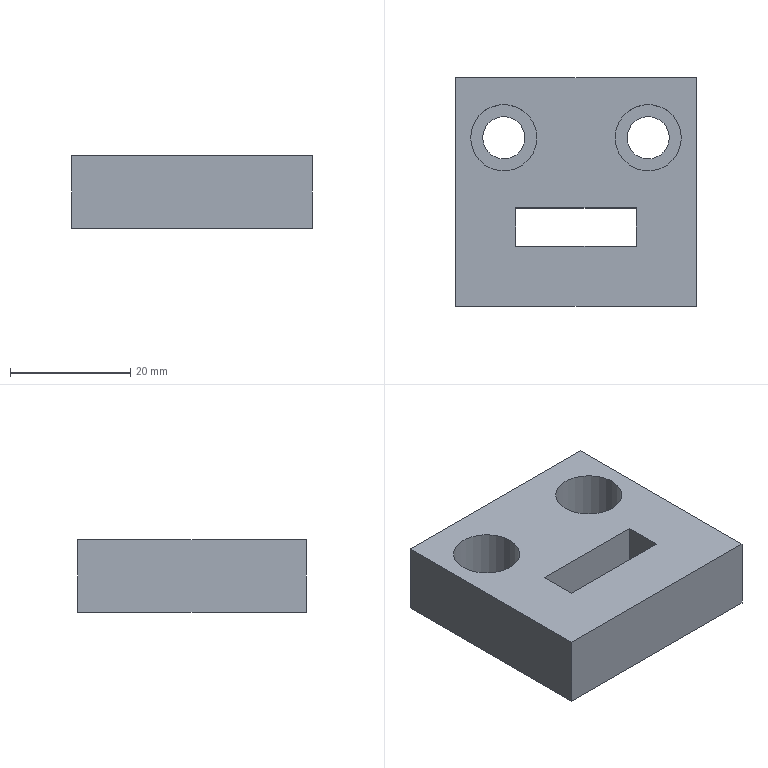Part | STEP file | lll_id714_x_t | 1 solid | 16 faces | box 40 x 38 x 12 mm | volume 14885 mm3 | plane 12 | cylinder 4 | commonest cylinder face diameters 7.009 x2 11.008 x2
STEP:
#1=CARTESIAN_POINT('',(295.5,-162.325,-12.));
#2=VERTEX_POINT('',#1);
#3=CARTESIAN_POINT('',(295.5,-168.675,-12.));
#4=VERTEX_POINT('',#3);
#5=CARTESIAN_POINT('',(295.5,-162.325,-12.));
#6=DIRECTION('',(0.,-1.,0.));
#7=VECTOR('',#6,1.);
#8=LINE('',#5,#7);
#9=EDGE_CURVE('',#2,#4,#8,.T.);
#10=ORIENTED_EDGE('',*,*,#9,.F.);
#11=CARTESIAN_POINT('',(275.5,-162.325,-12.));
#12=VERTEX_POINT('',#11);
#13=CARTESIAN_POINT('',(295.5,-162.325,-12.));
#14=DIRECTION('',(-1.,0.,0.));
#15=VECTOR('',#14,1.);
#16=LINE('',#13,#15);
#17=EDGE_CURVE('',#2,#12,#16,.T.);
#18=ORIENTED_EDGE('',*,*,#17,.T.);
#19=CARTESIAN_POINT('',(275.5,-168.675,-12.));
#20=VERTEX_POINT('',#19);
#21=CARTESIAN_POINT('',(275.5,-162.325,-12.));
#22=DIRECTION('',(0.,-1.,0.));
#23=VECTOR('',#22,1.);
#24=LINE('',#21,#23);
#25=EDGE_CURVE('',#12,#20,#24,.T.);
#26=ORIENTED_EDGE('',*,*,#25,.T.);
#27=CARTESIAN_POINT('',(295.5,-168.675,-12.));
#28=DIRECTION('',(-1.,0.,0.));
#29=VECTOR('',#28,1.);
#30=LINE('',#27,#29);
#31=EDGE_CURVE('',#4,#20,#30,.T.);
#32=ORIENTED_EDGE('',*,*,#31,.F.);
#33=EDGE_LOOP('',(#10,#18,#26,#32));
#34=FACE_BOUND('',#33,.T.);
#35=CARTESIAN_POINT('',(305.505,-140.675,-12.));
#36=VERTEX_POINT('',#35);
#37=CARTESIAN_POINT('',(305.505,-178.675,-12.));
#38=VERTEX_POINT('',#37);
#39=CARTESIAN_POINT('',(305.505,-165.5,-12.));
#40=DIRECTION('',(0.,-1.,0.));
#41=VECTOR('',#40,1.);
#42=LINE('',#39,#41);
#43=EDGE_CURVE('',#36,#38,#42,.T.);
#44=ORIENTED_EDGE('',*,*,#43,.T.);
#45=CARTESIAN_POINT('',(265.505,-178.675,-12.));
#46=VERTEX_POINT('',#45);
#47=CARTESIAN_POINT('',(0.,-178.675,-12.));
#48=DIRECTION('',(-1.,0.,0.));
#49=VECTOR('',#48,1.);
#50=LINE('',#47,#49);
#51=EDGE_CURVE('',#38,#46,#50,.T.);
#52=ORIENTED_EDGE('',*,*,#51,.T.);
#53=CARTESIAN_POINT('',(265.505,-140.675,-12.));
#54=VERTEX_POINT('',#53);
#55=CARTESIAN_POINT('',(265.505,-165.5,-12.));
#56=DIRECTION('',(0.,1.,0.));
#57=VECTOR('',#56,1.);
#58=LINE('',#55,#57);
#59=EDGE_CURVE('',#46,#54,#58,.T.);
#60=ORIENTED_EDGE('',*,*,#59,.T.);
#61=CARTESIAN_POINT('',(0.,-140.675,-12.));
#62=DIRECTION('',(1.,0.,0.));
#63=VECTOR('',#62,1.);
#64=LINE('',#61,#63);
#65=EDGE_CURVE('',#54,#36,#64,.T.);
#66=ORIENTED_EDGE('',*,*,#65,.T.);
#67=EDGE_LOOP('',(#44,#52,#60,#66));
#68=FACE_BOUND('',#67,.T.);
#69=CARTESIAN_POINT('',(277.009,-150.675,-12.));
#70=VERTEX_POINT('',#69);
#71=CARTESIAN_POINT('',(273.505,-150.675,-12.));
#72=DIRECTION('',(0.,0.,1.));
#73=DIRECTION('',(1.,0.,0.));
#74=AXIS2_PLACEMENT_3D('',#71,#72,#73);
#75=CIRCLE('',#74,3.505);
#76=EDGE_CURVE('',#70,#70,#75,.T.);
#77=ORIENTED_EDGE('',*,*,#76,.T.);
#78=EDGE_LOOP('',(#77));
#79=FACE_BOUND('',#78,.T.);
#80=CARTESIAN_POINT('',(294.,-150.675,-12.));
#81=VERTEX_POINT('',#80);
#82=CARTESIAN_POINT('',(297.505,-150.675,-12.));
#83=DIRECTION('',(0.,0.,-1.));
#84=DIRECTION('',(-1.,0.,0.));
#85=AXIS2_PLACEMENT_3D('',#82,#83,#84);
#86=CIRCLE('',#85,3.505);
#87=EDGE_CURVE('',#81,#81,#86,.T.);
#88=ORIENTED_EDGE('',*,*,#87,.F.);
#89=EDGE_LOOP('',(#88));
#90=FACE_BOUND('',#89,.T.);
#91=CARTESIAN_POINT('',(285.505,-165.5,-12.));
#92=DIRECTION('',(0.,0.,-1.));
#93=DIRECTION('',(1.,0.,0.));
#94=AXIS2_PLACEMENT_3D('',#91,#92,#93);
#95=PLANE('',#94);
#96=ADVANCED_FACE('',(#34,#68,#79,#90),#95,.T.);
#97=CARTESIAN_POINT('',(305.505,-140.675,0.));
#98=VERTEX_POINT('',#97);
#99=CARTESIAN_POINT('',(265.505,-140.675,0.));
#100=VERTEX_POINT('',#99);
#101=CARTESIAN_POINT('',(0.,-140.675,0.));
#102=DIRECTION('',(-1.,0.,0.));
#103=VECTOR('',#102,1.);
#104=LINE('',#101,#103);
#105=EDGE_CURVE('',#98,#100,#104,.T.);
#106=ORIENTED_EDGE('',*,*,#105,.T.);
#107=CARTESIAN_POINT('',(265.505,-178.675,0.));
#108=VERTEX_POINT('',#107);
#109=CARTESIAN_POINT('',(265.505,-165.5,0.));
#110=DIRECTION('',(0.,-1.,0.));
#111=VECTOR('',#110,1.);
#112=LINE('',#109,#111);
#113=EDGE_CURVE('',#100,#108,#112,.T.);
#114=ORIENTED_EDGE('',*,*,#113,.T.);
#115=CARTESIAN_POINT('',(305.505,-178.675,0.));
#116=VERTEX_POINT('',#115);
#117=CARTESIAN_POINT('',(0.,-178.675,0.));
#118=DIRECTION('',(1.,0.,0.));
#119=VECTOR('',#118,1.);
#120=LINE('',#117,#119);
#121=EDGE_CURVE('',#108,#116,#120,.T.);
#122=ORIENTED_EDGE('',*,*,#121,.T.);
#123=CARTESIAN_POINT('',(305.505,-165.5,0.));
#124=DIRECTION('',(0.,1.,0.));
#125=VECTOR('',#124,1.);
#126=LINE('',#123,#125);
#127=EDGE_CURVE('',#116,#98,#126,.T.);
#128=ORIENTED_EDGE('',*,*,#127,.T.);
#129=EDGE_LOOP('',(#106,#114,#122,#128));
#130=FACE_BOUND('',#129,.T.);
#131=CARTESIAN_POINT('',(295.5,-168.675,0.));
#132=VERTEX_POINT('',#131);
#133=CARTESIAN_POINT('',(275.5,-168.675,0.));
#134=VERTEX_POINT('',#133);
#135=CARTESIAN_POINT('',(295.5,-168.675,0.));
#136=DIRECTION('',(-1.,0.,0.));
#137=VECTOR('',#136,1.);
#138=LINE('',#135,#137);
#139=EDGE_CURVE('',#132,#134,#138,.T.);
#140=ORIENTED_EDGE('',*,*,#139,.T.);
#141=CARTESIAN_POINT('',(275.5,-162.325,0.));
#142=VERTEX_POINT('',#141);
#143=CARTESIAN_POINT('',(275.5,-162.325,0.));
#144=DIRECTION('',(0.,-1.,0.));
#145=VECTOR('',#144,1.);
#146=LINE('',#143,#145);
#147=EDGE_CURVE('',#142,#134,#146,.T.);
#148=ORIENTED_EDGE('',*,*,#147,.F.);
#149=CARTESIAN_POINT('',(295.5,-162.325,0.));
#150=VERTEX_POINT('',#149);
#151=CARTESIAN_POINT('',(295.5,-162.325,0.));
#152=DIRECTION('',(-1.,0.,0.));
#153=VECTOR('',#152,1.);
#154=LINE('',#151,#153);
#155=EDGE_CURVE('',#150,#142,#154,.T.);
#156=ORIENTED_EDGE('',*,*,#155,.F.);
#157=CARTESIAN_POINT('',(295.5,-162.325,0.));
#158=DIRECTION('',(0.,-1.,0.));
#159=VECTOR('',#158,1.);
#160=LINE('',#157,#159);
#161=EDGE_CURVE('',#150,#132,#160,.T.);
#162=ORIENTED_EDGE('',*,*,#161,.T.);
#163=EDGE_LOOP('',(#140,#148,#156,#162));
#164=FACE_BOUND('',#163,.T.);
#165=CARTESIAN_POINT('',(279.009,-150.675,0.));
#166=VERTEX_POINT('',#165);
#167=CARTESIAN_POINT('',(273.505,-150.675,0.));
#168=DIRECTION('',(0.,0.,-1.));
#169=DIRECTION('',(1.,0.,0.));
#170=AXIS2_PLACEMENT_3D('',#167,#168,#169);
#171=CIRCLE('',#170,5.504);
#172=EDGE_CURVE('',#166,#166,#171,.T.);
#173=ORIENTED_EDGE('',*,*,#172,.T.);
#174=EDGE_LOOP('',(#173));
#175=FACE_BOUND('',#174,.T.);
#176=CARTESIAN_POINT('',(292.001,-150.675,0.));
#177=VERTEX_POINT('',#176);
#178=CARTESIAN_POINT('',(297.505,-150.675,0.));
#179=DIRECTION('',(0.,0.,1.));
#180=DIRECTION('',(-1.,0.,0.));
#181=AXIS2_PLACEMENT_3D('',#178,#179,#180);
#182=CIRCLE('',#181,5.504);
#183=EDGE_CURVE('',#177,#177,#182,.T.);
#184=ORIENTED_EDGE('',*,*,#183,.F.);
#185=EDGE_LOOP('',(#184));
#186=FACE_BOUND('',#185,.T.);
#187=CARTESIAN_POINT('',(285.505,-165.5,0.));
#188=DIRECTION('',(0.,0.,1.));
#189=DIRECTION('',(-1.,0.,0.));
#190=AXIS2_PLACEMENT_3D('',#187,#188,#189);
#191=PLANE('',#190);
#192=ADVANCED_FACE('',(#130,#164,#175,#186),#191,.T.);
#193=CARTESIAN_POINT('',(305.505,-140.675,0.));
#194=DIRECTION('',(0.,0.,1.));
#195=VECTOR('',#194,1.);
#196=LINE('',#193,#195);
#197=EDGE_CURVE('',#36,#98,#196,.T.);
#198=ORIENTED_EDGE('',*,*,#197,.F.);
#199=ORIENTED_EDGE('',*,*,#65,.F.);
#200=CARTESIAN_POINT('',(265.505,-140.675,-12.));
#201=DIRECTION('',(0.,0.,1.));
#202=VECTOR('',#201,1.);
#203=LINE('',#200,#202);
#204=EDGE_CURVE('',#54,#100,#203,.T.);
#205=ORIENTED_EDGE('',*,*,#204,.T.);
#206=ORIENTED_EDGE('',*,*,#105,.F.);
#207=EDGE_LOOP('',(#198,#199,#205,#206));
#208=FACE_OUTER_BOUND('',#207,.T.);
#209=CARTESIAN_POINT('',(0.,-140.675,0.));
#210=DIRECTION('',(0.,1.,0.));
#211=DIRECTION('',(0.,0.,1.));
#212=AXIS2_PLACEMENT_3D('',#209,#210,#211);
#213=PLANE('',#212);
#214=ADVANCED_FACE('',(#208),#213,.T.);
#215=ORIENTED_EDGE('',*,*,#204,.F.);
#216=ORIENTED_EDGE('',*,*,#59,.F.);
#217=CARTESIAN_POINT('',(265.505,-178.675,0.));
#218=DIRECTION('',(0.,0.,1.));
#219=VECTOR('',#218,1.);
#220=LINE('',#217,#219);
#221=EDGE_CURVE('',#46,#108,#220,.T.);
#222=ORIENTED_EDGE('',*,*,#221,.T.);
#223=ORIENTED_EDGE('',*,*,#113,.F.);
#224=EDGE_LOOP('',(#215,#216,#222,#223));
#225=FACE_OUTER_BOUND('',#224,.T.);
#226=CARTESIAN_POINT('',(265.505,-165.5,-12.));
#227=DIRECTION('',(-1.,0.,0.));
#228=DIRECTION('',(0.,0.,-1.));
#229=AXIS2_PLACEMENT_3D('',#226,#227,#228);
#230=PLANE('',#229);
#231=ADVANCED_FACE('',(#225),#230,.T.);
#232=ORIENTED_EDGE('',*,*,#221,.F.);
#233=ORIENTED_EDGE('',*,*,#51,.F.);
#234=CARTESIAN_POINT('',(305.505,-178.675,-12.));
#235=DIRECTION('',(0.,0.,1.));
#236=VECTOR('',#235,1.);
#237=LINE('',#234,#236);
#238=EDGE_CURVE('',#38,#116,#237,.T.);
#239=ORIENTED_EDGE('',*,*,#238,.T.);
#240=ORIENTED_EDGE('',*,*,#121,.F.);
#241=EDGE_LOOP('',(#232,#233,#239,#240));
#242=FACE_OUTER_BOUND('',#241,.T.);
#243=CARTESIAN_POINT('',(0.,-178.675,0.));
#244=DIRECTION('',(0.,1.,0.));
#245=DIRECTION('',(0.,0.,1.));
#246=AXIS2_PLACEMENT_3D('',#243,#244,#245);
#247=PLANE('',#246);
#248=ADVANCED_FACE('',(#242),#247,.F.);
#249=ORIENTED_EDGE('',*,*,#43,.F.);
#250=ORIENTED_EDGE('',*,*,#197,.T.);
#251=ORIENTED_EDGE('',*,*,#127,.F.);
#252=ORIENTED_EDGE('',*,*,#238,.F.);
#253=EDGE_LOOP('',(#249,#250,#251,#252));
#254=FACE_OUTER_BOUND('',#253,.T.);
#255=CARTESIAN_POINT('',(305.505,-165.5,-12.));
#256=DIRECTION('',(1.,0.,0.));
#257=DIRECTION('',(0.,0.,1.));
#258=AXIS2_PLACEMENT_3D('',#255,#256,#257);
#259=PLANE('',#258);
#260=ADVANCED_FACE('',(#254),#259,.T.);
#261=CARTESIAN_POINT('',(275.5,-168.675,-12.));
#262=DIRECTION('',(0.,0.,-1.));
#263=VECTOR('',#262,1.);
#264=LINE('',#261,#263);
#265=EDGE_CURVE('',#134,#20,#264,.T.);
#266=ORIENTED_EDGE('',*,*,#265,.T.);
#267=ORIENTED_EDGE('',*,*,#25,.F.);
#268=CARTESIAN_POINT('',(275.5,-162.325,-12.));
#269=DIRECTION('',(0.,0.,-1.));
#270=VECTOR('',#269,1.);
#271=LINE('',#268,#270);
#272=EDGE_CURVE('',#142,#12,#271,.T.);
#273=ORIENTED_EDGE('',*,*,#272,.F.);
#274=ORIENTED_EDGE('',*,*,#147,.T.);
#275=EDGE_LOOP('',(#266,#267,#273,#274));
#276=FACE_OUTER_BOUND('',#275,.T.);
#277=CARTESIAN_POINT('',(275.5,-162.325,-12.));
#278=DIRECTION('',(-1.,0.,0.));
#279=DIRECTION('',(0.,0.,-1.));
#280=AXIS2_PLACEMENT_3D('',#277,#278,#279);
#281=PLANE('',#280);
#282=ADVANCED_FACE('',(#276),#281,.F.);
#283=CARTESIAN_POINT('',(295.5,-168.675,-12.));
#284=DIRECTION('',(0.,0.,-1.));
#285=VECTOR('',#284,1.);
#286=LINE('',#283,#285);
#287=EDGE_CURVE('',#132,#4,#286,.T.);
#288=ORIENTED_EDGE('',*,*,#287,.F.);
#289=ORIENTED_EDGE('',*,*,#161,.F.);
#290=CARTESIAN_POINT('',(295.5,-162.325,-12.));
#291=DIRECTION('',(0.,0.,-1.));
#292=VECTOR('',#291,1.);
#293=LINE('',#290,#292);
#294=EDGE_CURVE('',#150,#2,#293,.T.);
#295=ORIENTED_EDGE('',*,*,#294,.T.);
#296=ORIENTED_EDGE('',*,*,#9,.T.);
#297=EDGE_LOOP('',(#288,#289,#295,#296));
#298=FACE_OUTER_BOUND('',#297,.T.);
#299=CARTESIAN_POINT('',(295.5,-162.325,-12.));
#300=DIRECTION('',(-1.,0.,0.));
#301=DIRECTION('',(0.,0.,-1.));
#302=AXIS2_PLACEMENT_3D('',#299,#300,#301);
#303=PLANE('',#302);
#304=ADVANCED_FACE('',(#298),#303,.T.);
#305=ORIENTED_EDGE('',*,*,#272,.T.);
#306=ORIENTED_EDGE('',*,*,#17,.F.);
#307=ORIENTED_EDGE('',*,*,#294,.F.);
#308=ORIENTED_EDGE('',*,*,#155,.T.);
#309=EDGE_LOOP('',(#305,#306,#307,#308));
#310=FACE_OUTER_BOUND('',#309,.T.);
#311=CARTESIAN_POINT('',(0.,-162.325,0.));
#312=DIRECTION('',(0.,1.,0.));
#313=DIRECTION('',(0.,0.,1.));
#314=AXIS2_PLACEMENT_3D('',#311,#312,#313);
#315=PLANE('',#314);
#316=ADVANCED_FACE('',(#310),#315,.F.);
#317=ORIENTED_EDGE('',*,*,#265,.F.);
#318=ORIENTED_EDGE('',*,*,#139,.F.);
#319=ORIENTED_EDGE('',*,*,#287,.T.);
#320=ORIENTED_EDGE('',*,*,#31,.T.);
#321=EDGE_LOOP('',(#317,#318,#319,#320));
#322=FACE_OUTER_BOUND('',#321,.T.);
#323=CARTESIAN_POINT('',(0.,-168.675,0.));
#324=DIRECTION('',(0.,1.,0.));
#325=DIRECTION('',(0.,0.,1.));
#326=AXIS2_PLACEMENT_3D('',#323,#324,#325);
#327=PLANE('',#326);
#328=ADVANCED_FACE('',(#322),#327,.T.);
#329=CARTESIAN_POINT('',(270.,-150.675,-8.));
#330=VERTEX_POINT('',#329);
#331=CARTESIAN_POINT('',(273.505,-150.675,-8.));
#332=DIRECTION('',(0.,0.,-1.));
#333=DIRECTION('',(-1.,0.,0.));
#334=AXIS2_PLACEMENT_3D('',#331,#332,#333);
#335=CIRCLE('',#334,3.505);
#336=EDGE_CURVE('',#330,#330,#335,.T.);
#337=ORIENTED_EDGE('',*,*,#336,.F.);
#338=EDGE_LOOP('',(#337));
#339=FACE_BOUND('',#338,.T.);
#340=ORIENTED_EDGE('',*,*,#76,.F.);
#341=EDGE_LOOP('',(#340));
#342=FACE_BOUND('',#341,.T.);
#343=CARTESIAN_POINT('',(273.505,-150.675,0.));
#344=DIRECTION('',(0.,0.,-1.));
#345=DIRECTION('',(-1.,0.,0.));
#346=AXIS2_PLACEMENT_3D('',#343,#344,#345);
#347=CYLINDRICAL_SURFACE('',#346,3.505);
#348=ADVANCED_FACE('',(#339,#342),#347,.F.);
#349=ORIENTED_EDGE('',*,*,#336,.T.);
#350=EDGE_LOOP('',(#349));
#351=FACE_BOUND('',#350,.T.);
#352=CARTESIAN_POINT('',(268.001,-150.675,-8.));
#353=VERTEX_POINT('',#352);
#354=CARTESIAN_POINT('',(273.505,-150.675,-8.));
#355=DIRECTION('',(0.,0.,-1.));
#356=DIRECTION('',(-1.,0.,0.));
#357=AXIS2_PLACEMENT_3D('',#354,#355,#356);
#358=CIRCLE('',#357,5.504);
#359=EDGE_CURVE('',#353,#353,#358,.T.);
#360=ORIENTED_EDGE('',*,*,#359,.F.);
#361=EDGE_LOOP('',(#360));
#362=FACE_BOUND('',#361,.T.);
#363=CARTESIAN_POINT('',(273.505,-150.675,-8.));
#364=DIRECTION('',(0.,0.,-1.));
#365=DIRECTION('',(-1.,0.,0.));
#366=AXIS2_PLACEMENT_3D('',#363,#364,#365);
#367=PLANE('',#366);
#368=ADVANCED_FACE('',(#351,#362),#367,.F.);
#369=ORIENTED_EDGE('',*,*,#359,.T.);
#370=EDGE_LOOP('',(#369));
#371=FACE_BOUND('',#370,.T.);
#372=ORIENTED_EDGE('',*,*,#172,.F.);
#373=EDGE_LOOP('',(#372));
#374=FACE_BOUND('',#373,.T.);
#375=CARTESIAN_POINT('',(273.505,-150.675,0.));
#376=DIRECTION('',(0.,0.,-1.));
#377=DIRECTION('',(-1.,0.,0.));
#378=AXIS2_PLACEMENT_3D('',#375,#376,#377);
#379=CYLINDRICAL_SURFACE('',#378,5.504);
#380=ADVANCED_FACE('',(#371,#374),#379,.F.);
#381=CARTESIAN_POINT('',(294.,-150.675,-8.));
#382=VERTEX_POINT('',#381);
#383=CARTESIAN_POINT('',(297.505,-150.675,-8.));
#384=DIRECTION('',(0.,0.,1.));
#385=DIRECTION('',(-1.,0.,0.));
#386=AXIS2_PLACEMENT_3D('',#383,#384,#385);
#387=CIRCLE('',#386,3.505);
#388=EDGE_CURVE('',#382,#382,#387,.T.);
#389=ORIENTED_EDGE('',*,*,#388,.T.);
#390=EDGE_LOOP('',(#389));
#391=FACE_BOUND('',#390,.T.);
#392=ORIENTED_EDGE('',*,*,#87,.T.);
#393=EDGE_LOOP('',(#392));
#394=FACE_BOUND('',#393,.T.);
#395=CARTESIAN_POINT('',(297.505,-150.675,0.));
#396=DIRECTION('',(0.,0.,-1.));
#397=DIRECTION('',(1.,0.,0.));
#398=AXIS2_PLACEMENT_3D('',#395,#396,#397);
#399=CYLINDRICAL_SURFACE('',#398,3.505);
#400=ADVANCED_FACE('',(#391,#394),#399,.F.);
#401=ORIENTED_EDGE('',*,*,#388,.F.);
#402=EDGE_LOOP('',(#401));
#403=FACE_BOUND('',#402,.T.);
#404=CARTESIAN_POINT('',(292.001,-150.675,-8.));
#405=VERTEX_POINT('',#404);
#406=CARTESIAN_POINT('',(297.505,-150.675,-8.));
#407=DIRECTION('',(0.,0.,1.));
#408=DIRECTION('',(-1.,0.,0.));
#409=AXIS2_PLACEMENT_3D('',#406,#407,#408);
#410=CIRCLE('',#409,5.504);
#411=EDGE_CURVE('',#405,#405,#410,.T.);
#412=ORIENTED_EDGE('',*,*,#411,.T.);
#413=EDGE_LOOP('',(#412));
#414=FACE_BOUND('',#413,.T.);
#415=CARTESIAN_POINT('',(297.505,-150.675,-8.));
#416=DIRECTION('',(0.,0.,-1.));
#417=DIRECTION('',(1.,0.,0.));
#418=AXIS2_PLACEMENT_3D('',#415,#416,#417);
#419=PLANE('',#418);
#420=ADVANCED_FACE('',(#403,#414),#419,.F.);
#421=ORIENTED_EDGE('',*,*,#411,.F.);
#422=EDGE_LOOP('',(#421));
#423=FACE_BOUND('',#422,.T.);
#424=ORIENTED_EDGE('',*,*,#183,.T.);
#425=EDGE_LOOP('',(#424));
#426=FACE_BOUND('',#425,.T.);
#427=CARTESIAN_POINT('',(297.505,-150.675,0.));
#428=DIRECTION('',(0.,0.,-1.));
#429=DIRECTION('',(1.,0.,0.));
#430=AXIS2_PLACEMENT_3D('',#427,#428,#429);
#431=CYLINDRICAL_SURFACE('',#430,5.504);
#432=ADVANCED_FACE('',(#423,#426),#431,.F.);
#433=CLOSED_SHELL('',(#96,#192,#214,#231,#248,#260,#282,#304,#316,#328,#348,#368,#380,#400,#420,#432));
#434=MANIFOLD_SOLID_BREP('',#433);
#435=(LENGTH_UNIT()NAMED_UNIT(*)SI_UNIT(.MILLI.,.METRE.));
#436=UNCERTAINTY_MEASURE_WITH_UNIT(LENGTH_MEASURE(0.00002),#435,'','');
#437=(NAMED_UNIT(*)PLANE_ANGLE_UNIT()SI_UNIT($,.RADIAN.));
#438=PLANE_ANGLE_MEASURE_WITH_UNIT(PLANE_ANGLE_MEASURE(0.01745),#437);
#439=DIMENSIONAL_EXPONENTS(0.,0.,0.,0.,0.,0.,0.);
#440=(CONVERSION_BASED_UNIT('DEGREE',#438)NAMED_UNIT(#439)PLANE_ANGLE_UNIT());
#441=(NAMED_UNIT(*)SI_UNIT($,.STERADIAN.)SOLID_ANGLE_UNIT());
#442=(GEOMETRIC_REPRESENTATION_CONTEXT(3)GLOBAL_UNCERTAINTY_ASSIGNED_CONTEXT((#436))GLOBAL_UNIT_ASSIGNED_CONTEXT((#435,#440,#441))REPRESENTATION_CONTEXT('',''));
#443=ADVANCED_BREP_SHAPE_REPRESENTATION('',(#434),#442);